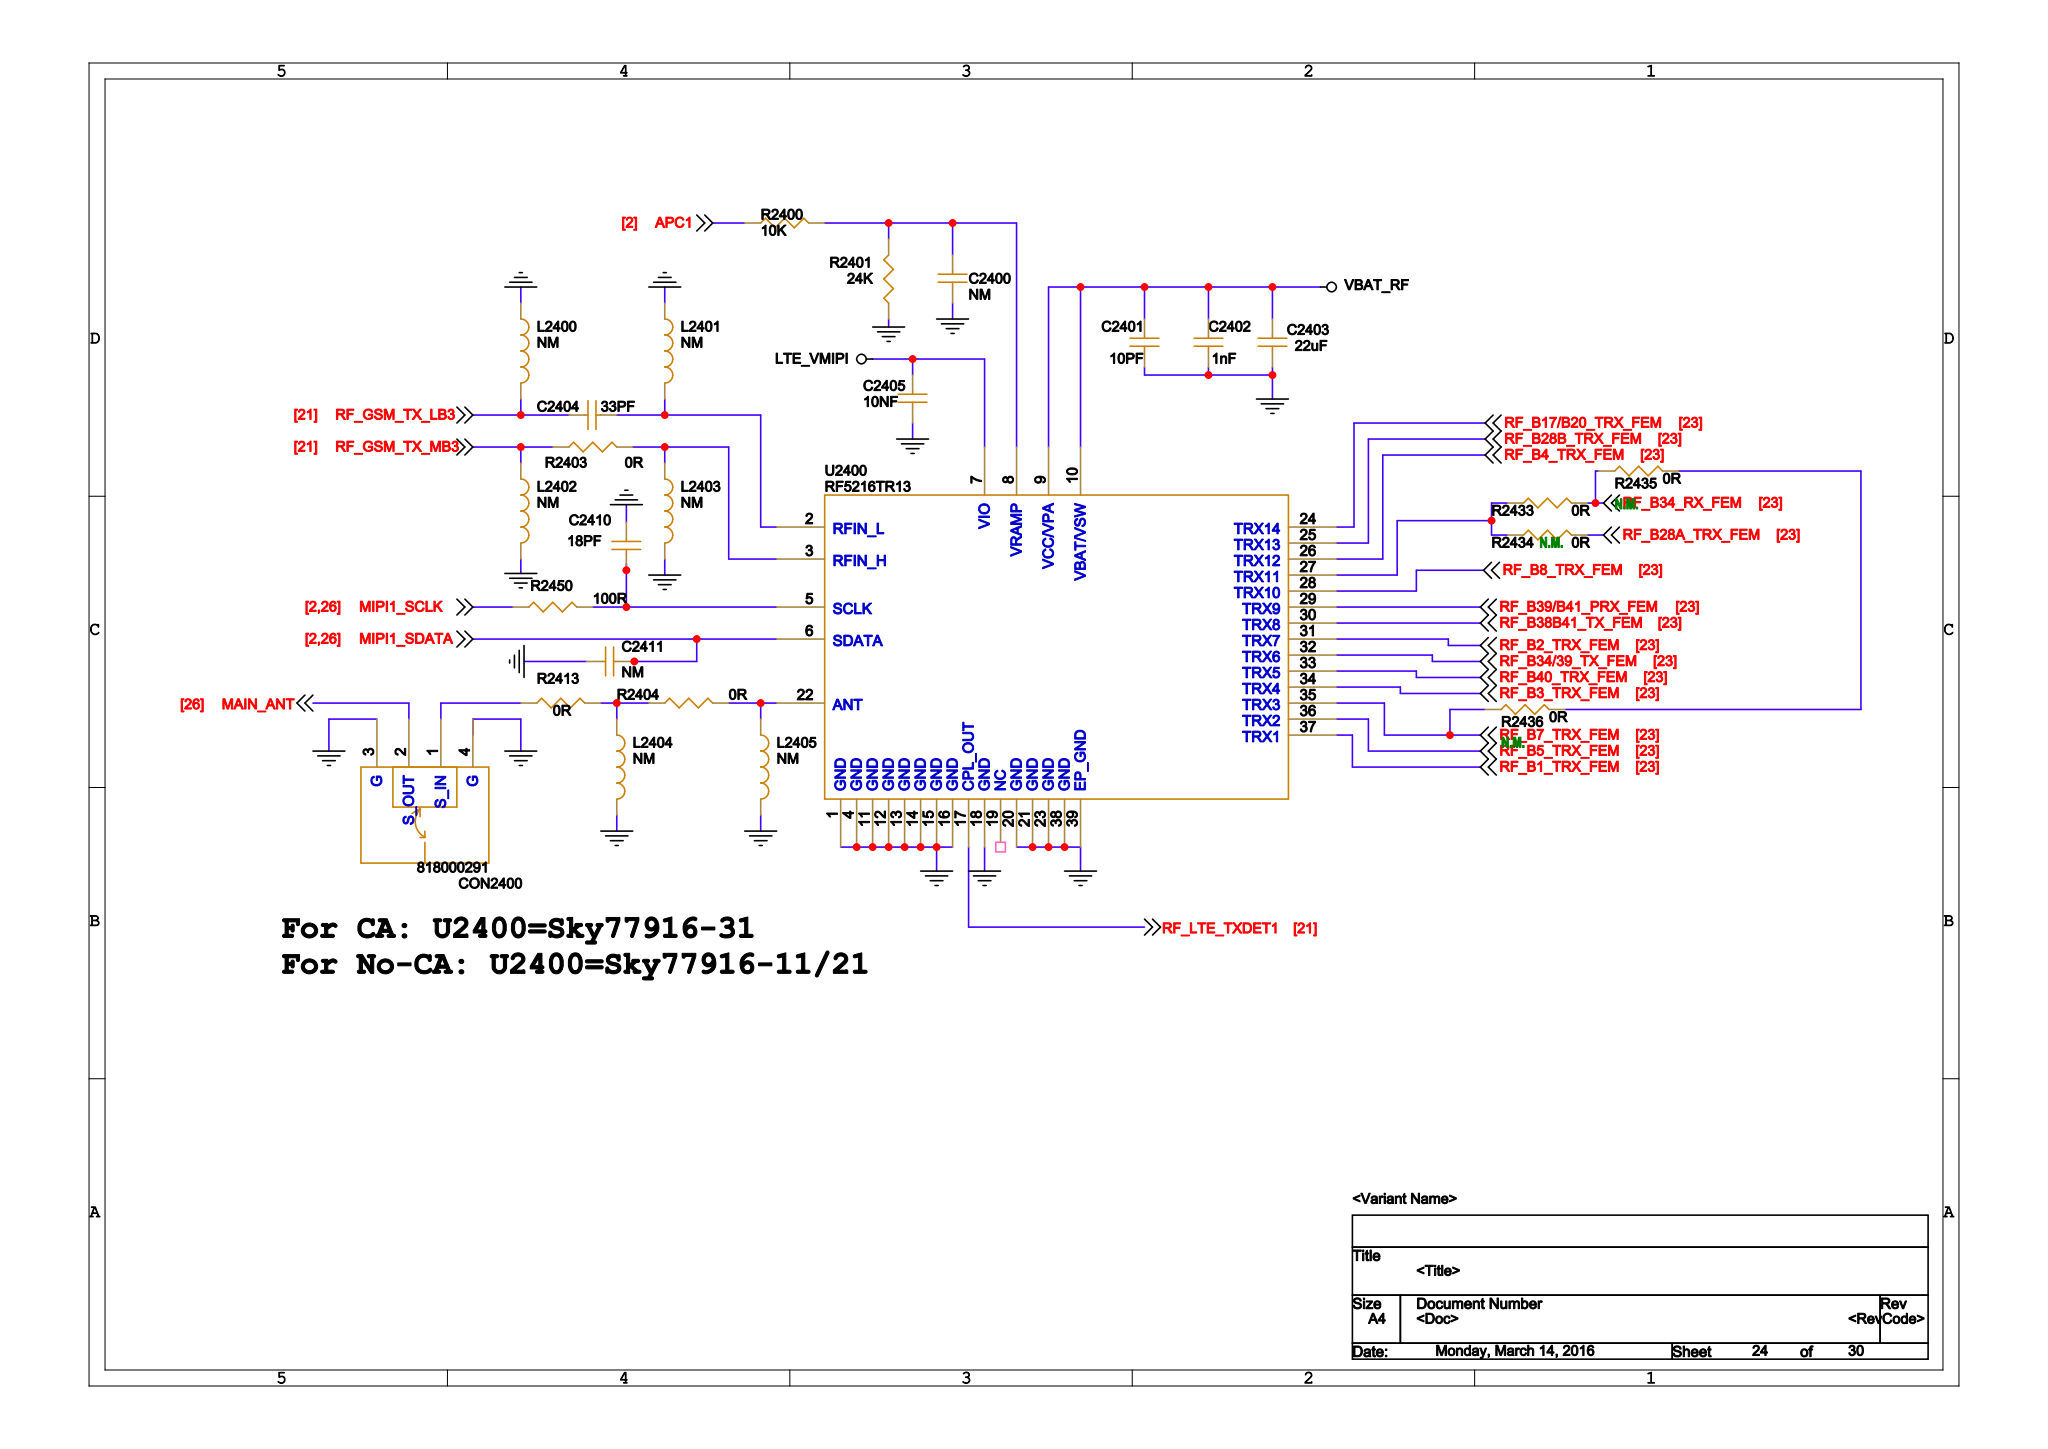Circuit board | Cadence Allegro | 1088 parts | 793 nets | one sheet of the schematic
Parts on this sheet (reference | value | footprint):
C2400 | NM | 0201_NM
C2401 | 10PF | C0201
C2402 | 1nF | C0201
C2403 | 22uF | 0402-BIG
C2404 | 33PF | C0201
C2405 | 10nF | C0201
C2410 | 18PF | C0201
C2411 | NM | 0201_NM
CON2400 | 818000291 | RF_818000291
L2400 | NM | 0201_NM
L2401 | NM | 0201_NM
L2402 | NM | 0201_NM
L2403 | NM | 0201_NM
L2404 | NM | 0201_NM
L2405 | NM | 0201_NM
R2400 | 10K | R0201
R2401 | 24K | R0201
R2403 | 0R | R0201
R2404 | 0R | R0201
R2413 | 0R | R0201
R2433 | 0R | R0201
R2434
R2435
R2436
R2450 | 100R | R0201
U2400 | RF5216TR13 | RF5216
Nets of these parts (net: part-pin ...):
GND: C2400-2 C2401-2 C2402-2 C2403-2 C2405-2 C2410-1 C2411-1 CON2400-3 CON2400-4 L2400-1 L2401-1 L2402-2 L2403-2 L2404-2 L2405-2 R2401-2 U2400-1 U2400-4 U2400-11 U2400-12 U2400-13 U2400-14 U2400-15 U2400-16 U2400-18 U2400-20 U2400-21 U2400-23 U2400-38 U2400-39
MIPI1_SCLK: R2450-1
MIPI1_SDATA: C2411-2 U2400-6
N33455731: CON2400-1 R2413-1
MAIN_ANT: CON2400-2
APC1: R2400-2
VBAT_RF: C2401-1 C2402-1 C2403-1 U2400-9 U2400-10
LTE_VMIPI: C2405-1 U2400-7
N31361261: L2405-1 R2404-2 U2400-22
RF_LTE_TXDET1: U2400-17
N31360319: L2403-1 R2403-2 U2400-3
N31360155: C2404-2 L2401-2 U2400-2
N35645173: C2410-2 R2450-2 U2400-5
RF_B1_TRX_FEM: U2400-37
RF_B8_TRX_FEM: U2400-28
N33455726: R2433-1 R2434-1 U2400-27
RF_B4_TRX_FEM: U2400-26
RF_B28B_TRX_FEM: U2400-25
RF_B17/B20_TRX_FEM: U2400-24
RF_B5_TRX_FEM: U2400-36
RF_B7_TRX_FEM: R2436-1 U2400-35
RF_B3_TRX_FEM: U2400-34
RF_B40_TRX_FEM: U2400-33
RF_B34/39_TX_FEM: U2400-32
RF_B2_TRX_FEM: U2400-31
RF_B38B41_TX_FEM: U2400-30
RF_B39/B41_PRX_FEM: U2400-29
N31362607: C2400-1 R2400-1 R2401-1 U2400-8
RF_GSM_TX_LB3: C2404-1 L2400-2
RF_GSM_TX_MB3: L2402-1 R2403-1
N32482417: L2404-1 R2404-1 R2413-2
RF_B34_RX_FEM: R2433-2 R2435-1
RF_B28A_TRX_FEM: R2434-2
N34624731: R2435-2 R2436-2